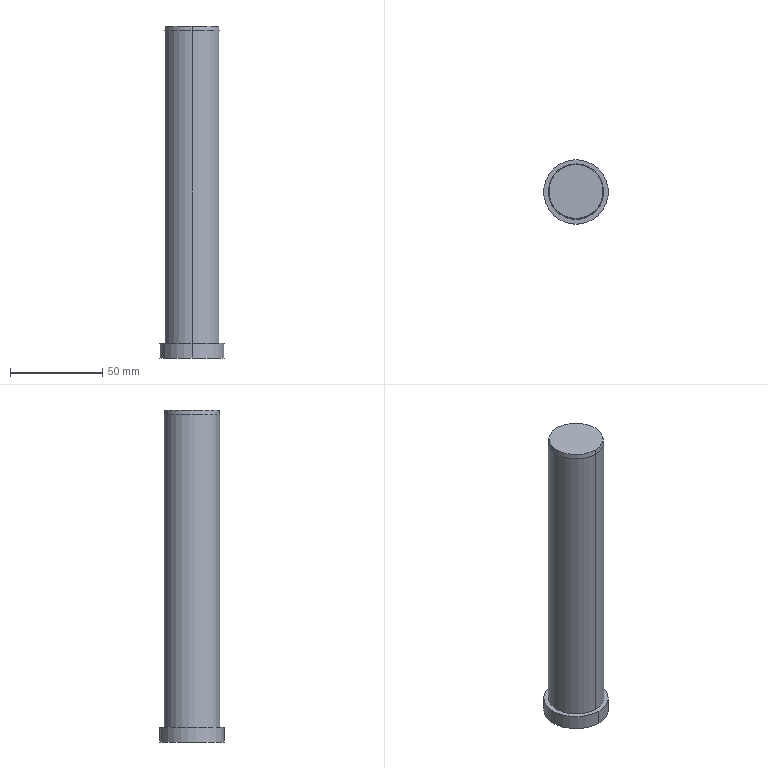Part | Creo | 1 solid | 16 faces | box 35 x 35 x 180 mm | volume 127760 mm3 | cylinder 8 | plane 4 | cone 4 | commonest cylinder face diameters 10.5 x2 12 x2 30 x2 35 x2
STEP:
#1=CARTESIAN_POINT('',(145.,195.311,-186.));
#2=VERTEX_POINT('',#1);
#3=CARTESIAN_POINT('',(145.,224.68,-186.));
#4=VERTEX_POINT('',#3);
#5=CARTESIAN_POINT('',(145.,209.995,-186.));
#6=DIRECTION('',(0.,0.,1.));
#7=DIRECTION('',(0.,-1.,0.));
#8=AXIS2_PLACEMENT_3D('',#5,#6,#7);
#9=CIRCLE('',#8,14.684);
#10=EDGE_CURVE('',#2,#4,#9,.T.);
#11=ORIENTED_EDGE('',*,*,#10,.F.);
#12=CARTESIAN_POINT('',(145.,209.995,-186.));
#13=DIRECTION('',(0.,0.,1.));
#14=DIRECTION('',(0.,1.,0.));
#15=AXIS2_PLACEMENT_3D('',#12,#13,#14);
#16=CIRCLE('',#15,14.684);
#17=EDGE_CURVE('',#4,#2,#16,.T.);
#18=ORIENTED_EDGE('',*,*,#17,.F.);
#19=EDGE_LOOP('',(#11,#18));
#20=FACE_OUTER_BOUND('',#19,.F.);
#21=CARTESIAN_POINT('',(145.,209.995,-186.));
#22=DIRECTION('',(0.,0.,-1.));
#23=DIRECTION('',(0.,-1.,0.));
#24=AXIS2_PLACEMENT_3D('',#21,#22,#23);
#25=PLANE('',#24);
#26=ADVANCED_FACE('',(#20),#25,.F.);
#27=ORIENTED_EDGE('',*,*,#10,.T.);
#28=CARTESIAN_POINT('',(145.,224.995,-188.57));
#29=VERTEX_POINT('',#28);
#30=CARTESIAN_POINT('',(145.,224.68,-186.));
#31=DIRECTION('',(0.,0.1219,-0.9925));
#32=VECTOR('',#31,2.589);
#33=LINE('',#30,#32);
#34=EDGE_CURVE('',#4,#29,#33,.T.);
#35=ORIENTED_EDGE('',*,*,#34,.T.);
#36=CARTESIAN_POINT('',(145.,194.995,-188.57));
#37=VERTEX_POINT('',#36);
#38=CARTESIAN_POINT('',(145.,209.995,-188.57));
#39=DIRECTION('',(0.,0.,1.));
#40=DIRECTION('',(0.,-1.,0.));
#41=AXIS2_PLACEMENT_3D('',#38,#39,#40);
#42=CIRCLE('',#41,15.);
#43=EDGE_CURVE('',#37,#29,#42,.T.);
#44=ORIENTED_EDGE('',*,*,#43,.F.);
#45=CARTESIAN_POINT('',(145.,195.311,-186.));
#46=DIRECTION('',(0.,-0.1219,-0.9925));
#47=VECTOR('',#46,2.589);
#48=LINE('',#45,#47);
#49=EDGE_CURVE('',#2,#37,#48,.T.);
#50=ORIENTED_EDGE('',*,*,#49,.F.);
#51=EDGE_LOOP('',(#27,#35,#44,#50));
#52=FACE_OUTER_BOUND('',#51,.F.);
#53=CARTESIAN_POINT('',(145.,209.995,-187.285));
#54=DIRECTION('',(0.,0.,-1.));
#55=DIRECTION('',(0.,-1.,0.));
#56=AXIS2_PLACEMENT_3D('',#53,#54,#55);
#57=CONICAL_SURFACE('',#56,14.842,7.);
#58=ADVANCED_FACE('',(#52),#57,.T.);
#59=ORIENTED_EDGE('',*,*,#17,.T.);
#60=ORIENTED_EDGE('',*,*,#49,.T.);
#61=CARTESIAN_POINT('',(145.,209.995,-188.57));
#62=DIRECTION('',(0.,0.,1.));
#63=DIRECTION('',(0.,1.,0.));
#64=AXIS2_PLACEMENT_3D('',#61,#62,#63);
#65=CIRCLE('',#64,15.);
#66=EDGE_CURVE('',#29,#37,#65,.T.);
#67=ORIENTED_EDGE('',*,*,#66,.F.);
#68=ORIENTED_EDGE('',*,*,#34,.F.);
#69=EDGE_LOOP('',(#59,#60,#67,#68));
#70=FACE_OUTER_BOUND('',#69,.F.);
#71=CARTESIAN_POINT('',(145.,209.995,-187.285));
#72=DIRECTION('',(0.,0.,-1.));
#73=DIRECTION('',(0.,-1.,0.));
#74=AXIS2_PLACEMENT_3D('',#71,#72,#73);
#75=CONICAL_SURFACE('',#74,14.842,7.);
#76=ADVANCED_FACE('',(#70),#75,.T.);
#77=CARTESIAN_POINT('',(145.,194.995,-358.));
#78=VERTEX_POINT('',#77);
#79=CARTESIAN_POINT('',(145.,224.995,-358.));
#80=VERTEX_POINT('',#79);
#81=CARTESIAN_POINT('',(145.,209.995,-358.));
#82=DIRECTION('',(0.,0.,-1.));
#83=DIRECTION('',(0.,-1.,0.));
#84=AXIS2_PLACEMENT_3D('',#81,#82,#83);
#85=CIRCLE('',#84,15.);
#86=EDGE_CURVE('',#78,#80,#85,.T.);
#87=ORIENTED_EDGE('',*,*,#86,.T.);
#88=CARTESIAN_POINT('',(145.,224.995,-188.57));
#89=DIRECTION('',(0.,0.,-1.));
#90=VECTOR('',#89,169.43);
#91=LINE('',#88,#90);
#92=EDGE_CURVE('',#29,#80,#91,.T.);
#93=ORIENTED_EDGE('',*,*,#92,.F.);
#94=ORIENTED_EDGE('',*,*,#66,.T.);
#95=CARTESIAN_POINT('',(145.,194.995,-188.57));
#96=DIRECTION('',(0.,0.,-1.));
#97=VECTOR('',#96,169.43);
#98=LINE('',#95,#97);
#99=EDGE_CURVE('',#37,#78,#98,.T.);
#100=ORIENTED_EDGE('',*,*,#99,.T.);
#101=EDGE_LOOP('',(#87,#93,#94,#100));
#102=FACE_OUTER_BOUND('',#101,.F.);
#103=CARTESIAN_POINT('',(145.,209.995,-173.5));
#104=DIRECTION('',(0.,0.,-1.));
#105=DIRECTION('',(0.,-1.,0.));
#106=AXIS2_PLACEMENT_3D('',#103,#104,#105);
#107=CYLINDRICAL_SURFACE('',#106,15.);
#108=ADVANCED_FACE('',(#102),#107,.T.);
#109=CARTESIAN_POINT('',(145.,192.495,-358.));
#110=VERTEX_POINT('',#109);
#111=CARTESIAN_POINT('',(145.,227.495,-358.));
#112=VERTEX_POINT('',#111);
#113=CARTESIAN_POINT('',(145.,209.995,-358.));
#114=DIRECTION('',(0.,0.,1.));
#115=DIRECTION('',(0.,-1.,0.));
#116=AXIS2_PLACEMENT_3D('',#113,#114,#115);
#117=CIRCLE('',#116,17.5);
#118=EDGE_CURVE('',#110,#112,#117,.T.);
#119=ORIENTED_EDGE('',*,*,#118,.F.);
#120=CARTESIAN_POINT('',(145.,209.995,-358.));
#121=DIRECTION('',(0.,0.,1.));
#122=DIRECTION('',(0.,1.,0.));
#123=AXIS2_PLACEMENT_3D('',#120,#121,#122);
#124=CIRCLE('',#123,17.5);
#125=EDGE_CURVE('',#112,#110,#124,.T.);
#126=ORIENTED_EDGE('',*,*,#125,.F.);
#127=EDGE_LOOP('',(#119,#126));
#128=FACE_OUTER_BOUND('',#127,.F.);
#129=ORIENTED_EDGE('',*,*,#86,.F.);
#130=CARTESIAN_POINT('',(145.,209.995,-358.));
#131=DIRECTION('',(0.,0.,-1.));
#132=DIRECTION('',(0.,1.,0.));
#133=AXIS2_PLACEMENT_3D('',#130,#131,#132);
#134=CIRCLE('',#133,15.);
#135=EDGE_CURVE('',#80,#78,#134,.T.);
#136=ORIENTED_EDGE('',*,*,#135,.F.);
#137=EDGE_LOOP('',(#129,#136));
#138=FACE_BOUND('',#137,.F.);
#139=CARTESIAN_POINT('',(145.,209.995,-358.));
#140=DIRECTION('',(0.,0.,1.));
#141=DIRECTION('',(0.,1.,0.));
#142=AXIS2_PLACEMENT_3D('',#139,#140,#141);
#143=PLANE('',#142);
#144=ADVANCED_FACE('',(#128,#138),#143,.T.);
#145=ORIENTED_EDGE('',*,*,#135,.T.);
#146=ORIENTED_EDGE('',*,*,#99,.F.);
#147=ORIENTED_EDGE('',*,*,#43,.T.);
#148=ORIENTED_EDGE('',*,*,#92,.T.);
#149=EDGE_LOOP('',(#145,#146,#147,#148));
#150=FACE_OUTER_BOUND('',#149,.F.);
#151=CARTESIAN_POINT('',(145.,209.995,-173.5));
#152=DIRECTION('',(0.,0.,-1.));
#153=DIRECTION('',(0.,-1.,0.));
#154=AXIS2_PLACEMENT_3D('',#151,#152,#153);
#155=CYLINDRICAL_SURFACE('',#154,15.);
#156=ADVANCED_FACE('',(#150),#155,.T.);
#157=ORIENTED_EDGE('',*,*,#118,.T.);
#158=CARTESIAN_POINT('',(145.,227.495,-366.));
#159=VERTEX_POINT('',#158);
#160=CARTESIAN_POINT('',(145.,227.495,-366.));
#161=DIRECTION('',(0.,0.,1.));
#162=VECTOR('',#161,8.);
#163=LINE('',#160,#162);
#164=EDGE_CURVE('',#159,#112,#163,.T.);
#165=ORIENTED_EDGE('',*,*,#164,.F.);
#166=CARTESIAN_POINT('',(145.,192.495,-366.));
#167=VERTEX_POINT('',#166);
#168=CARTESIAN_POINT('',(145.,209.995,-366.));
#169=DIRECTION('',(0.,0.,-1.));
#170=DIRECTION('',(0.,1.,0.));
#171=AXIS2_PLACEMENT_3D('',#168,#169,#170);
#172=CIRCLE('',#171,17.5);
#173=EDGE_CURVE('',#159,#167,#172,.T.);
#174=ORIENTED_EDGE('',*,*,#173,.T.);
#175=CARTESIAN_POINT('',(145.,192.495,-366.));
#176=DIRECTION('',(0.,0.,1.));
#177=VECTOR('',#176,8.);
#178=LINE('',#175,#177);
#179=EDGE_CURVE('',#167,#110,#178,.T.);
#180=ORIENTED_EDGE('',*,*,#179,.T.);
#181=EDGE_LOOP('',(#157,#165,#174,#180));
#182=FACE_OUTER_BOUND('',#181,.F.);
#183=CARTESIAN_POINT('',(145.,209.995,-366.4));
#184=DIRECTION('',(0.,0.,1.));
#185=DIRECTION('',(0.,1.,0.));
#186=AXIS2_PLACEMENT_3D('',#183,#184,#185);
#187=CYLINDRICAL_SURFACE('',#186,17.5);
#188=ADVANCED_FACE('',(#182),#187,.T.);
#189=ORIENTED_EDGE('',*,*,#125,.T.);
#190=ORIENTED_EDGE('',*,*,#179,.F.);
#191=CARTESIAN_POINT('',(145.,209.995,-366.));
#192=DIRECTION('',(0.,0.,-1.));
#193=DIRECTION('',(0.,-1.,0.));
#194=AXIS2_PLACEMENT_3D('',#191,#192,#193);
#195=CIRCLE('',#194,17.5);
#196=EDGE_CURVE('',#167,#159,#195,.T.);
#197=ORIENTED_EDGE('',*,*,#196,.T.);
#198=ORIENTED_EDGE('',*,*,#164,.T.);
#199=EDGE_LOOP('',(#189,#190,#197,#198));
#200=FACE_OUTER_BOUND('',#199,.F.);
#201=CARTESIAN_POINT('',(145.,209.995,-366.4));
#202=DIRECTION('',(0.,0.,1.));
#203=DIRECTION('',(0.,1.,0.));
#204=AXIS2_PLACEMENT_3D('',#201,#202,#203);
#205=CYLINDRICAL_SURFACE('',#204,17.5);
#206=ADVANCED_FACE('',(#200),#205,.T.);
#207=ORIENTED_EDGE('',*,*,#196,.F.);
#208=ORIENTED_EDGE('',*,*,#173,.F.);
#209=EDGE_LOOP('',(#207,#208));
#210=FACE_OUTER_BOUND('',#209,.F.);
#211=CARTESIAN_POINT('',(151.,209.995,-366.));
#212=VERTEX_POINT('',#211);
#213=CARTESIAN_POINT('',(139.,209.995,-366.));
#214=VERTEX_POINT('',#213);
#215=CARTESIAN_POINT('',(145.,209.995,-366.));
#216=DIRECTION('',(0.,0.,1.));
#217=DIRECTION('',(1.,0.,0.));
#218=AXIS2_PLACEMENT_3D('',#215,#216,#217);
#219=CIRCLE('',#218,6.);
#220=EDGE_CURVE('',#212,#214,#219,.T.);
#221=ORIENTED_EDGE('',*,*,#220,.F.);
#222=CARTESIAN_POINT('',(145.,209.995,-366.));
#223=DIRECTION('',(0.,0.,1.));
#224=DIRECTION('',(-1.,0.,0.));
#225=AXIS2_PLACEMENT_3D('',#222,#223,#224);
#226=CIRCLE('',#225,6.);
#227=EDGE_CURVE('',#214,#212,#226,.T.);
#228=ORIENTED_EDGE('',*,*,#227,.F.);
#229=EDGE_LOOP('',(#221,#228));
#230=FACE_BOUND('',#229,.F.);
#231=CARTESIAN_POINT('',(145.,209.995,-366.));
#232=DIRECTION('',(0.,0.,-1.));
#233=DIRECTION('',(0.,-1.,0.));
#234=AXIS2_PLACEMENT_3D('',#231,#232,#233);
#235=PLANE('',#234);
#236=ADVANCED_FACE('',(#210,#230),#235,.T.);
#237=ORIENTED_EDGE('',*,*,#220,.T.);
#238=CARTESIAN_POINT('',(139.,209.995,-356.));
#239=VERTEX_POINT('',#238);
#240=CARTESIAN_POINT('',(139.,209.995,-366.));
#241=DIRECTION('',(0.,0.,1.));
#242=VECTOR('',#241,10.);
#243=LINE('',#240,#242);
#244=EDGE_CURVE('',#214,#239,#243,.T.);
#245=ORIENTED_EDGE('',*,*,#244,.T.);
#246=CARTESIAN_POINT('',(151.,209.995,-356.));
#247=VERTEX_POINT('',#246);
#248=CARTESIAN_POINT('',(145.,209.995,-356.));
#249=DIRECTION('',(0.,0.,-1.));
#250=DIRECTION('',(-1.,0.,0.));
#251=AXIS2_PLACEMENT_3D('',#248,#249,#250);
#252=CIRCLE('',#251,6.);
#253=EDGE_CURVE('',#239,#247,#252,.T.);
#254=ORIENTED_EDGE('',*,*,#253,.T.);
#255=CARTESIAN_POINT('',(151.,209.995,-366.));
#256=DIRECTION('',(0.,0.,1.));
#257=VECTOR('',#256,10.);
#258=LINE('',#255,#257);
#259=EDGE_CURVE('',#212,#247,#258,.T.);
#260=ORIENTED_EDGE('',*,*,#259,.F.);
#261=EDGE_LOOP('',(#237,#245,#254,#260));
#262=FACE_OUTER_BOUND('',#261,.F.);
#263=CARTESIAN_POINT('',(145.,209.995,-391.));
#264=DIRECTION('',(0.,0.,1.));
#265=DIRECTION('',(1.,0.,0.));
#266=AXIS2_PLACEMENT_3D('',#263,#264,#265);
#267=CYLINDRICAL_SURFACE('',#266,6.);
#268=ADVANCED_FACE('',(#262),#267,.F.);
#269=ORIENTED_EDGE('',*,*,#227,.T.);
#270=ORIENTED_EDGE('',*,*,#259,.T.);
#271=CARTESIAN_POINT('',(145.,209.995,-356.));
#272=DIRECTION('',(0.,0.,-1.));
#273=DIRECTION('',(1.,0.,0.));
#274=AXIS2_PLACEMENT_3D('',#271,#272,#273);
#275=CIRCLE('',#274,6.);
#276=EDGE_CURVE('',#247,#239,#275,.T.);
#277=ORIENTED_EDGE('',*,*,#276,.T.);
#278=ORIENTED_EDGE('',*,*,#244,.F.);
#279=EDGE_LOOP('',(#269,#270,#277,#278));
#280=FACE_OUTER_BOUND('',#279,.F.);
#281=CARTESIAN_POINT('',(145.,209.995,-391.));
#282=DIRECTION('',(0.,0.,1.));
#283=DIRECTION('',(1.,0.,0.));
#284=AXIS2_PLACEMENT_3D('',#281,#282,#283);
#285=CYLINDRICAL_SURFACE('',#284,6.);
#286=ADVANCED_FACE('',(#280),#285,.F.);
#287=ORIENTED_EDGE('',*,*,#276,.F.);
#288=ORIENTED_EDGE('',*,*,#253,.F.);
#289=EDGE_LOOP('',(#287,#288));
#290=FACE_OUTER_BOUND('',#289,.F.);
#291=CARTESIAN_POINT('',(150.25,209.995,-356.));
#292=VERTEX_POINT('',#291);
#293=CARTESIAN_POINT('',(139.75,209.995,-356.));
#294=VERTEX_POINT('',#293);
#295=CARTESIAN_POINT('',(145.,209.995,-356.));
#296=DIRECTION('',(0.,0.,1.));
#297=DIRECTION('',(1.,0.,0.));
#298=AXIS2_PLACEMENT_3D('',#295,#296,#297);
#299=CIRCLE('',#298,5.25);
#300=EDGE_CURVE('',#292,#294,#299,.T.);
#301=ORIENTED_EDGE('',*,*,#300,.F.);
#302=CARTESIAN_POINT('',(145.,209.995,-356.));
#303=DIRECTION('',(0.,0.,1.));
#304=DIRECTION('',(-1.,0.,0.));
#305=AXIS2_PLACEMENT_3D('',#302,#303,#304);
#306=CIRCLE('',#305,5.25);
#307=EDGE_CURVE('',#294,#292,#306,.T.);
#308=ORIENTED_EDGE('',*,*,#307,.F.);
#309=EDGE_LOOP('',(#301,#308));
#310=FACE_BOUND('',#309,.F.);
#311=CARTESIAN_POINT('',(145.,209.995,-356.));
#312=DIRECTION('',(0.,0.,1.));
#313=DIRECTION('',(1.,0.,0.));
#314=AXIS2_PLACEMENT_3D('',#311,#312,#313);
#315=PLANE('',#314);
#316=ADVANCED_FACE('',(#290,#310),#315,.F.);
#317=ORIENTED_EDGE('',*,*,#300,.T.);
#318=CARTESIAN_POINT('',(139.75,209.995,-353.));
#319=VERTEX_POINT('',#318);
#320=CARTESIAN_POINT('',(139.75,209.995,-356.));
#321=DIRECTION('',(0.,0.,1.));
#322=VECTOR('',#321,3.);
#323=LINE('',#320,#322);
#324=EDGE_CURVE('',#294,#319,#323,.T.);
#325=ORIENTED_EDGE('',*,*,#324,.T.);
#326=CARTESIAN_POINT('',(150.25,209.995,-353.));
#327=VERTEX_POINT('',#326);
#328=CARTESIAN_POINT('',(145.,209.995,-353.));
#329=DIRECTION('',(0.,0.,-1.));
#330=DIRECTION('',(-1.,0.,0.));
#331=AXIS2_PLACEMENT_3D('',#328,#329,#330);
#332=CIRCLE('',#331,5.25);
#333=EDGE_CURVE('',#319,#327,#332,.T.);
#334=ORIENTED_EDGE('',*,*,#333,.T.);
#335=CARTESIAN_POINT('',(150.25,209.995,-356.));
#336=DIRECTION('',(0.,0.,1.));
#337=VECTOR('',#336,3.);
#338=LINE('',#335,#337);
#339=EDGE_CURVE('',#292,#327,#338,.T.);
#340=ORIENTED_EDGE('',*,*,#339,.F.);
#341=EDGE_LOOP('',(#317,#325,#334,#340));
#342=FACE_OUTER_BOUND('',#341,.F.);
#343=CARTESIAN_POINT('',(145.,209.995,-391.));
#344=DIRECTION('',(0.,0.,1.));
#345=DIRECTION('',(1.,0.,0.));
#346=AXIS2_PLACEMENT_3D('',#343,#344,#345);
#347=CYLINDRICAL_SURFACE('',#346,5.25);
#348=ADVANCED_FACE('',(#342),#347,.F.);
#349=ORIENTED_EDGE('',*,*,#307,.T.);
#350=ORIENTED_EDGE('',*,*,#339,.T.);
#351=CARTESIAN_POINT('',(145.,209.995,-353.));
#352=DIRECTION('',(0.,0.,-1.));
#353=DIRECTION('',(1.,0.,0.));
#354=AXIS2_PLACEMENT_3D('',#351,#352,#353);
#355=CIRCLE('',#354,5.25);
#356=EDGE_CURVE('',#327,#319,#355,.T.);
#357=ORIENTED_EDGE('',*,*,#356,.T.);
#358=ORIENTED_EDGE('',*,*,#324,.F.);
#359=EDGE_LOOP('',(#349,#350,#357,#358));
#360=FACE_OUTER_BOUND('',#359,.F.);
#361=CARTESIAN_POINT('',(145.,209.995,-391.));
#362=DIRECTION('',(0.,0.,1.));
#363=DIRECTION('',(1.,0.,0.));
#364=AXIS2_PLACEMENT_3D('',#361,#362,#363);
#365=CYLINDRICAL_SURFACE('',#364,5.25);
#366=ADVANCED_FACE('',(#360),#365,.F.);
#367=ORIENTED_EDGE('',*,*,#356,.F.);
#368=CARTESIAN_POINT('',(145.,209.995,-349.969));
#369=VERTEX_POINT('',#368);
#370=CARTESIAN_POINT('',(145.,209.995,-349.969));
#371=DIRECTION('',(0.866,0.,-0.5));
#372=VECTOR('',#371,6.062);
#373=LINE('',#370,#372);
#374=EDGE_CURVE('',#369,#327,#373,.T.);
#375=ORIENTED_EDGE('',*,*,#374,.F.);
#376=CARTESIAN_POINT('',(145.,209.995,-349.969));
#377=DIRECTION('',(-0.866,0.,-0.5));
#378=VECTOR('',#377,6.062);
#379=LINE('',#376,#378);
#380=EDGE_CURVE('',#369,#319,#379,.T.);
#381=ORIENTED_EDGE('',*,*,#380,.T.);
#382=EDGE_LOOP('',(#367,#375,#381));
#383=FACE_OUTER_BOUND('',#382,.F.);
#384=CARTESIAN_POINT('',(145.,209.995,-351.54));
#385=DIRECTION('',(0.,0.,-1.));
#386=DIRECTION('',(-1.,0.,0.));
#387=AXIS2_PLACEMENT_3D('',#384,#385,#386);
#388=CONICAL_SURFACE('',#387,2.722,60.);
#389=ADVANCED_FACE('',(#383),#388,.F.);
#390=ORIENTED_EDGE('',*,*,#333,.F.);
#391=ORIENTED_EDGE('',*,*,#380,.F.);
#392=ORIENTED_EDGE('',*,*,#374,.T.);
#393=EDGE_LOOP('',(#390,#391,#392));
#394=FACE_OUTER_BOUND('',#393,.F.);
#395=CARTESIAN_POINT('',(145.,209.995,-351.54));
#396=DIRECTION('',(0.,0.,-1.));
#397=DIRECTION('',(-1.,0.,0.));
#398=AXIS2_PLACEMENT_3D('',#395,#396,#397);
#399=CONICAL_SURFACE('',#398,2.722,60.);
#400=ADVANCED_FACE('',(#394),#399,.F.);
#401=CLOSED_SHELL('',(#26,#58,#76,#108,#144,#156,#188,#206,#236,#268,#286,#316,#348,#366,#389,#400));
#402=MANIFOLD_SOLID_BREP('',#401);
#403=(LENGTH_UNIT()NAMED_UNIT(*)SI_UNIT(.MILLI.,.METRE.));
#404=UNCERTAINTY_MEASURE_WITH_UNIT(LENGTH_MEASURE(0.01867),#403,'','');
#405=(NAMED_UNIT(*)PLANE_ANGLE_UNIT()SI_UNIT($,.RADIAN.));
#406=PLANE_ANGLE_MEASURE_WITH_UNIT(PLANE_ANGLE_MEASURE(0.01745),#405);
#407=(CONVERSION_BASED_UNIT('DEGREE',#406)NAMED_UNIT(*)PLANE_ANGLE_UNIT());
#408=(NAMED_UNIT(*)SI_UNIT($,.STERADIAN.)SOLID_ANGLE_UNIT());
#409=(GEOMETRIC_REPRESENTATION_CONTEXT(3)GLOBAL_UNCERTAINTY_ASSIGNED_CONTEXT((#404))GLOBAL_UNIT_ASSIGNED_CONTEXT((#403,#407,#408))REPRESENTATION_CONTEXT('',''));
#410=ADVANCED_BREP_SHAPE_REPRESENTATION('',(#402),#409);